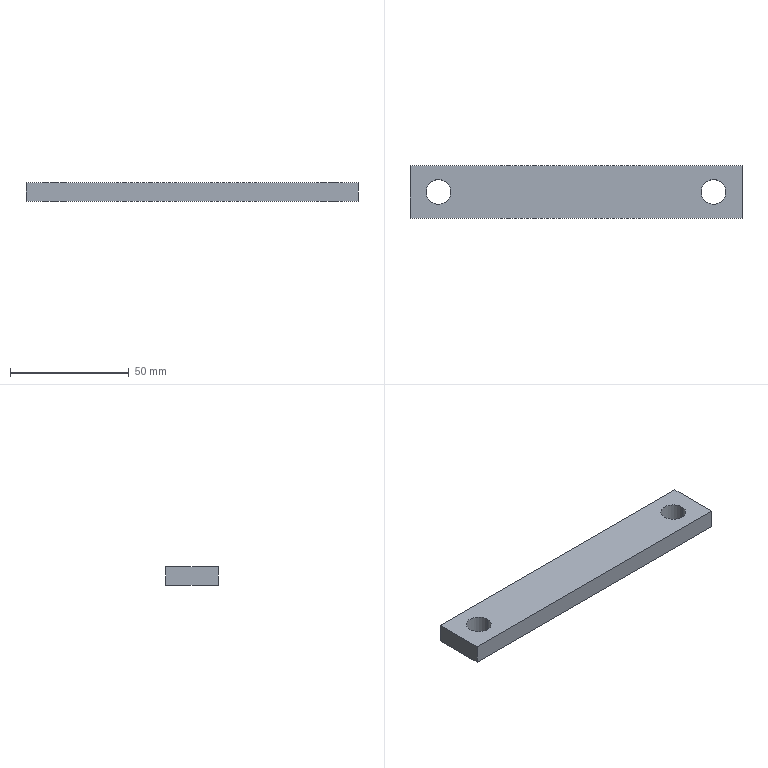Part | SolidWorks | features Extrusion 1, ICE 1 | 1 solid | 10 faces | box 140 x 22 x 8 mm | volume 23255 mm3 | plane 6 | cylinder 4 | commonest cylinder face diameters 10.5 x4
STEP:
#1=CARTESIAN_POINT('',(-63.16,24.003,0.));
#2=VERTEX_POINT('',#1);
#3=CARTESIAN_POINT('',(-52.66,24.003,0.));
#4=VERTEX_POINT('',#3);
#5=CARTESIAN_POINT('',(-57.91,24.003,0.));
#6=DIRECTION('',(0.,0.,1.));
#7=DIRECTION('',(1.,0.,0.));
#8=AXIS2_PLACEMENT_3D('',#5,#6,#7);
#9=CIRCLE('',#8,5.25);
#10=EDGE_CURVE('',#2,#4,#9,.T.);
#11=ORIENTED_EDGE('',*,*,#10,.F.);
#12=CARTESIAN_POINT('',(-63.16,24.003,8.));
#13=VERTEX_POINT('',#12);
#14=CARTESIAN_POINT('',(-63.16,24.003,0.));
#15=DIRECTION('',(0.,0.,1.));
#16=VECTOR('',#15,1000.);
#17=LINE('',#14,#16);
#18=EDGE_CURVE('',#2,#13,#17,.T.);
#19=ORIENTED_EDGE('',*,*,#18,.T.);
#20=CARTESIAN_POINT('',(-52.66,24.003,8.));
#21=VERTEX_POINT('',#20);
#22=CARTESIAN_POINT('',(-57.91,24.003,8.));
#23=DIRECTION('',(0.,0.,1.));
#24=DIRECTION('',(1.,0.,0.));
#25=AXIS2_PLACEMENT_3D('',#22,#23,#24);
#26=CIRCLE('',#25,5.25);
#27=EDGE_CURVE('',#13,#21,#26,.T.);
#28=ORIENTED_EDGE('',*,*,#27,.T.);
#29=CARTESIAN_POINT('',(-52.66,24.003,0.));
#30=DIRECTION('',(0.,0.,1.));
#31=VECTOR('',#30,1000.);
#32=LINE('',#29,#31);
#33=EDGE_CURVE('',#4,#21,#32,.T.);
#34=ORIENTED_EDGE('',*,*,#33,.F.);
#35=EDGE_LOOP('',(#11,#19,#28,#34));
#36=FACE_OUTER_BOUND('',#35,.T.);
#37=CARTESIAN_POINT('',(-57.91,24.003,0.));
#38=DIRECTION('',(0.,0.,1.));
#39=DIRECTION('',(1.,0.,0.));
#40=AXIS2_PLACEMENT_3D('',#37,#38,#39);
#41=CYLINDRICAL_SURFACE('',#40,5.25);
#42=ADVANCED_FACE('',(#36),#41,.F.);
#43=CARTESIAN_POINT('',(52.84,24.003,0.));
#44=VERTEX_POINT('',#43);
#45=CARTESIAN_POINT('',(63.34,24.003,0.));
#46=VERTEX_POINT('',#45);
#47=CARTESIAN_POINT('',(58.09,24.003,0.));
#48=DIRECTION('',(0.,0.,1.));
#49=DIRECTION('',(-1.,0.,0.));
#50=AXIS2_PLACEMENT_3D('',#47,#48,#49);
#51=CIRCLE('',#50,5.25);
#52=EDGE_CURVE('',#44,#46,#51,.T.);
#53=ORIENTED_EDGE('',*,*,#52,.F.);
#54=CARTESIAN_POINT('',(52.84,24.003,8.));
#55=VERTEX_POINT('',#54);
#56=CARTESIAN_POINT('',(52.84,24.003,0.));
#57=DIRECTION('',(0.,0.,1.));
#58=VECTOR('',#57,1000.);
#59=LINE('',#56,#58);
#60=EDGE_CURVE('',#44,#55,#59,.T.);
#61=ORIENTED_EDGE('',*,*,#60,.T.);
#62=CARTESIAN_POINT('',(63.34,24.003,8.));
#63=VERTEX_POINT('',#62);
#64=CARTESIAN_POINT('',(58.09,24.003,8.));
#65=DIRECTION('',(0.,0.,1.));
#66=DIRECTION('',(-1.,0.,0.));
#67=AXIS2_PLACEMENT_3D('',#64,#65,#66);
#68=CIRCLE('',#67,5.25);
#69=EDGE_CURVE('',#55,#63,#68,.T.);
#70=ORIENTED_EDGE('',*,*,#69,.T.);
#71=CARTESIAN_POINT('',(63.34,24.003,0.));
#72=DIRECTION('',(0.,0.,1.));
#73=VECTOR('',#72,1000.);
#74=LINE('',#71,#73);
#75=EDGE_CURVE('',#46,#63,#74,.T.);
#76=ORIENTED_EDGE('',*,*,#75,.F.);
#77=EDGE_LOOP('',(#53,#61,#70,#76));
#78=FACE_OUTER_BOUND('',#77,.T.);
#79=CARTESIAN_POINT('',(58.09,24.003,0.));
#80=DIRECTION('',(0.,0.,1.));
#81=DIRECTION('',(1.,0.,0.));
#82=AXIS2_PLACEMENT_3D('',#79,#80,#81);
#83=CYLINDRICAL_SURFACE('',#82,5.25);
#84=ADVANCED_FACE('',(#78),#83,.F.);
#85=CARTESIAN_POINT('',(-69.91,35.003,0.));
#86=VERTEX_POINT('',#85);
#87=CARTESIAN_POINT('',(-69.91,13.003,0.));
#88=VERTEX_POINT('',#87);
#89=CARTESIAN_POINT('',(-69.91,35.003,0.));
#90=DIRECTION('',(0.,-1.,0.));
#91=VECTOR('',#90,1000.);
#92=LINE('',#89,#91);
#93=EDGE_CURVE('',#86,#88,#92,.T.);
#94=ORIENTED_EDGE('',*,*,#93,.T.);
#95=CARTESIAN_POINT('',(-69.91,13.003,8.));
#96=VERTEX_POINT('',#95);
#97=CARTESIAN_POINT('',(-69.91,13.003,8.));
#98=DIRECTION('',(0.,0.,-1.));
#99=VECTOR('',#98,1000.);
#100=LINE('',#97,#99);
#101=EDGE_CURVE('',#96,#88,#100,.T.);
#102=ORIENTED_EDGE('',*,*,#101,.F.);
#103=CARTESIAN_POINT('',(-69.91,35.003,8.));
#104=VERTEX_POINT('',#103);
#105=CARTESIAN_POINT('',(-69.91,35.003,8.));
#106=DIRECTION('',(0.,-1.,0.));
#107=VECTOR('',#106,1000.);
#108=LINE('',#105,#107);
#109=EDGE_CURVE('',#104,#96,#108,.T.);
#110=ORIENTED_EDGE('',*,*,#109,.F.);
#111=CARTESIAN_POINT('',(-69.91,35.003,8.));
#112=DIRECTION('',(0.,0.,-1.));
#113=VECTOR('',#112,1000.);
#114=LINE('',#111,#113);
#115=EDGE_CURVE('',#104,#86,#114,.T.);
#116=ORIENTED_EDGE('',*,*,#115,.T.);
#117=EDGE_LOOP('',(#94,#102,#110,#116));
#118=FACE_OUTER_BOUND('',#117,.T.);
#119=CARTESIAN_POINT('',(-69.91,35.003,8.));
#120=DIRECTION('',(1.,0.,0.));
#121=DIRECTION('',(0.,0.,-1.));
#122=AXIS2_PLACEMENT_3D('',#119,#120,#121);
#123=PLANE('',#122);
#124=ADVANCED_FACE('',(#118),#123,.F.);
#125=CARTESIAN_POINT('',(70.09,13.003,0.));
#126=VERTEX_POINT('',#125);
#127=CARTESIAN_POINT('',(-69.91,13.003,0.));
#128=DIRECTION('',(1.,0.,0.));
#129=VECTOR('',#128,1000.);
#130=LINE('',#127,#129);
#131=EDGE_CURVE('',#88,#126,#130,.T.);
#132=ORIENTED_EDGE('',*,*,#131,.T.);
#133=CARTESIAN_POINT('',(70.09,13.003,8.));
#134=VERTEX_POINT('',#133);
#135=CARTESIAN_POINT('',(70.09,13.003,8.));
#136=DIRECTION('',(0.,0.,-1.));
#137=VECTOR('',#136,1000.);
#138=LINE('',#135,#137);
#139=EDGE_CURVE('',#134,#126,#138,.T.);
#140=ORIENTED_EDGE('',*,*,#139,.F.);
#141=CARTESIAN_POINT('',(-69.91,13.003,8.));
#142=DIRECTION('',(1.,0.,0.));
#143=VECTOR('',#142,1000.);
#144=LINE('',#141,#143);
#145=EDGE_CURVE('',#96,#134,#144,.T.);
#146=ORIENTED_EDGE('',*,*,#145,.F.);
#147=ORIENTED_EDGE('',*,*,#101,.T.);
#148=EDGE_LOOP('',(#132,#140,#146,#147));
#149=FACE_OUTER_BOUND('',#148,.T.);
#150=CARTESIAN_POINT('',(-69.91,13.003,8.));
#151=DIRECTION('',(0.,1.,0.));
#152=DIRECTION('',(0.,0.,1.));
#153=AXIS2_PLACEMENT_3D('',#150,#151,#152);
#154=PLANE('',#153);
#155=ADVANCED_FACE('',(#149),#154,.F.);
#156=CARTESIAN_POINT('',(70.09,35.003,0.));
#157=VERTEX_POINT('',#156);
#158=CARTESIAN_POINT('',(70.09,35.003,0.));
#159=DIRECTION('',(0.,1.,0.));
#160=VECTOR('',#159,1000.);
#161=LINE('',#158,#160);
#162=EDGE_CURVE('',#126,#157,#161,.T.);
#163=ORIENTED_EDGE('',*,*,#162,.T.);
#164=CARTESIAN_POINT('',(70.09,35.003,8.));
#165=VERTEX_POINT('',#164);
#166=CARTESIAN_POINT('',(70.09,35.003,8.));
#167=DIRECTION('',(0.,0.,-1.));
#168=VECTOR('',#167,1000.);
#169=LINE('',#166,#168);
#170=EDGE_CURVE('',#165,#157,#169,.T.);
#171=ORIENTED_EDGE('',*,*,#170,.F.);
#172=CARTESIAN_POINT('',(70.09,35.003,8.));
#173=DIRECTION('',(0.,1.,0.));
#174=VECTOR('',#173,1000.);
#175=LINE('',#172,#174);
#176=EDGE_CURVE('',#134,#165,#175,.T.);
#177=ORIENTED_EDGE('',*,*,#176,.F.);
#178=ORIENTED_EDGE('',*,*,#139,.T.);
#179=EDGE_LOOP('',(#163,#171,#177,#178));
#180=FACE_OUTER_BOUND('',#179,.T.);
#181=CARTESIAN_POINT('',(70.09,35.003,8.));
#182=DIRECTION('',(-1.,0.,0.));
#183=DIRECTION('',(0.,0.,1.));
#184=AXIS2_PLACEMENT_3D('',#181,#182,#183);
#185=PLANE('',#184);
#186=ADVANCED_FACE('',(#180),#185,.F.);
#187=CARTESIAN_POINT('',(-69.91,35.003,0.));
#188=DIRECTION('',(-1.,0.,0.));
#189=VECTOR('',#188,1000.);
#190=LINE('',#187,#189);
#191=EDGE_CURVE('',#157,#86,#190,.T.);
#192=ORIENTED_EDGE('',*,*,#191,.T.);
#193=ORIENTED_EDGE('',*,*,#115,.F.);
#194=CARTESIAN_POINT('',(-69.91,35.003,8.));
#195=DIRECTION('',(-1.,0.,0.));
#196=VECTOR('',#195,1000.);
#197=LINE('',#194,#196);
#198=EDGE_CURVE('',#165,#104,#197,.T.);
#199=ORIENTED_EDGE('',*,*,#198,.F.);
#200=ORIENTED_EDGE('',*,*,#170,.T.);
#201=EDGE_LOOP('',(#192,#193,#199,#200));
#202=FACE_OUTER_BOUND('',#201,.T.);
#203=CARTESIAN_POINT('',(-69.91,35.003,8.));
#204=DIRECTION('',(0.,-1.,0.));
#205=DIRECTION('',(0.,0.,-1.));
#206=AXIS2_PLACEMENT_3D('',#203,#204,#205);
#207=PLANE('',#206);
#208=ADVANCED_FACE('',(#202),#207,.F.);
#209=CARTESIAN_POINT('',(-57.91,24.003,8.));
#210=DIRECTION('',(0.,0.,1.));
#211=DIRECTION('',(1.,0.,0.));
#212=AXIS2_PLACEMENT_3D('',#209,#210,#211);
#213=CIRCLE('',#212,5.25);
#214=EDGE_CURVE('',#21,#13,#213,.T.);
#215=ORIENTED_EDGE('',*,*,#214,.F.);
#216=ORIENTED_EDGE('',*,*,#27,.F.);
#217=EDGE_LOOP('',(#215,#216));
#218=FACE_BOUND('',#217,.T.);
#219=CARTESIAN_POINT('',(58.09,24.003,8.));
#220=DIRECTION('',(0.,0.,1.));
#221=DIRECTION('',(-1.,0.,0.));
#222=AXIS2_PLACEMENT_3D('',#219,#220,#221);
#223=CIRCLE('',#222,5.25);
#224=EDGE_CURVE('',#63,#55,#223,.T.);
#225=ORIENTED_EDGE('',*,*,#224,.F.);
#226=ORIENTED_EDGE('',*,*,#69,.F.);
#227=EDGE_LOOP('',(#225,#226));
#228=FACE_BOUND('',#227,.T.);
#229=ORIENTED_EDGE('',*,*,#109,.T.);
#230=ORIENTED_EDGE('',*,*,#145,.T.);
#231=ORIENTED_EDGE('',*,*,#176,.T.);
#232=ORIENTED_EDGE('',*,*,#198,.T.);
#233=EDGE_LOOP('',(#229,#230,#231,#232));
#234=FACE_OUTER_BOUND('',#233,.T.);
#235=CARTESIAN_POINT('',(0.,0.,8.));
#236=DIRECTION('',(0.,0.,1.));
#237=DIRECTION('',(1.,0.,0.));
#238=AXIS2_PLACEMENT_3D('',#235,#236,#237);
#239=PLANE('',#238);
#240=ADVANCED_FACE('',(#218,#228,#234),#239,.T.);
#241=CARTESIAN_POINT('',(-57.91,24.003,0.));
#242=DIRECTION('',(0.,0.,1.));
#243=DIRECTION('',(1.,0.,0.));
#244=AXIS2_PLACEMENT_3D('',#241,#242,#243);
#245=CIRCLE('',#244,5.25);
#246=EDGE_CURVE('',#4,#2,#245,.T.);
#247=ORIENTED_EDGE('',*,*,#246,.T.);
#248=ORIENTED_EDGE('',*,*,#10,.T.);
#249=EDGE_LOOP('',(#247,#248));
#250=FACE_BOUND('',#249,.T.);
#251=CARTESIAN_POINT('',(58.09,24.003,0.));
#252=DIRECTION('',(0.,0.,1.));
#253=DIRECTION('',(-1.,0.,0.));
#254=AXIS2_PLACEMENT_3D('',#251,#252,#253);
#255=CIRCLE('',#254,5.25);
#256=EDGE_CURVE('',#46,#44,#255,.T.);
#257=ORIENTED_EDGE('',*,*,#256,.T.);
#258=ORIENTED_EDGE('',*,*,#52,.T.);
#259=EDGE_LOOP('',(#257,#258));
#260=FACE_BOUND('',#259,.T.);
#261=ORIENTED_EDGE('',*,*,#93,.F.);
#262=ORIENTED_EDGE('',*,*,#191,.F.);
#263=ORIENTED_EDGE('',*,*,#162,.F.);
#264=ORIENTED_EDGE('',*,*,#131,.F.);
#265=EDGE_LOOP('',(#261,#262,#263,#264));
#266=FACE_OUTER_BOUND('',#265,.T.);
#267=CARTESIAN_POINT('',(0.,0.,0.));
#268=DIRECTION('',(0.,0.,1.));
#269=DIRECTION('',(1.,0.,0.));
#270=AXIS2_PLACEMENT_3D('',#267,#268,#269);
#271=PLANE('',#270);
#272=ADVANCED_FACE('',(#250,#260,#266),#271,.F.);
#273=ORIENTED_EDGE('',*,*,#60,.F.);
#274=ORIENTED_EDGE('',*,*,#256,.F.);
#275=ORIENTED_EDGE('',*,*,#75,.T.);
#276=ORIENTED_EDGE('',*,*,#224,.T.);
#277=EDGE_LOOP('',(#273,#274,#275,#276));
#278=FACE_OUTER_BOUND('',#277,.T.);
#279=CARTESIAN_POINT('',(58.09,24.003,0.));
#280=DIRECTION('',(0.,0.,1.));
#281=DIRECTION('',(1.,0.,0.));
#282=AXIS2_PLACEMENT_3D('',#279,#280,#281);
#283=CYLINDRICAL_SURFACE('',#282,5.25);
#284=ADVANCED_FACE('',(#278),#283,.F.);
#285=ORIENTED_EDGE('',*,*,#18,.F.);
#286=ORIENTED_EDGE('',*,*,#246,.F.);
#287=ORIENTED_EDGE('',*,*,#33,.T.);
#288=ORIENTED_EDGE('',*,*,#214,.T.);
#289=EDGE_LOOP('',(#285,#286,#287,#288));
#290=FACE_OUTER_BOUND('',#289,.T.);
#291=CARTESIAN_POINT('',(-57.91,24.003,0.));
#292=DIRECTION('',(0.,0.,1.));
#293=DIRECTION('',(1.,0.,0.));
#294=AXIS2_PLACEMENT_3D('',#291,#292,#293);
#295=CYLINDRICAL_SURFACE('',#294,5.25);
#296=ADVANCED_FACE('',(#290),#295,.F.);
#297=CLOSED_SHELL('',(#42,#84,#124,#155,#186,#208,#240,#272,#284,#296));
#298=MANIFOLD_SOLID_BREP('',#297);
#299=CARTESIAN_POINT('',(0.,0.,0.));
#300=DIRECTION('',(0.,0.,1.));
#301=DIRECTION('',(1.,0.,0.));
#302=AXIS2_PLACEMENT_3D('',#299,#300,#301);
#303=(LENGTH_UNIT()NAMED_UNIT(*)SI_UNIT(.MILLI.,.METRE.));
#304=UNCERTAINTY_MEASURE_WITH_UNIT(LENGTH_MEASURE(0.00001),#303,'','');
#305=(NAMED_UNIT(*)PLANE_ANGLE_UNIT()SI_UNIT($,.RADIAN.));
#306=(NAMED_UNIT(*)SI_UNIT($,.STERADIAN.)SOLID_ANGLE_UNIT());
#307=(GEOMETRIC_REPRESENTATION_CONTEXT(3)GLOBAL_UNCERTAINTY_ASSIGNED_CONTEXT((#304))GLOBAL_UNIT_ASSIGNED_CONTEXT((#303,#305,#306))REPRESENTATION_CONTEXT('',''));
#308=ADVANCED_BREP_SHAPE_REPRESENTATION('',(#298,#302),#307);